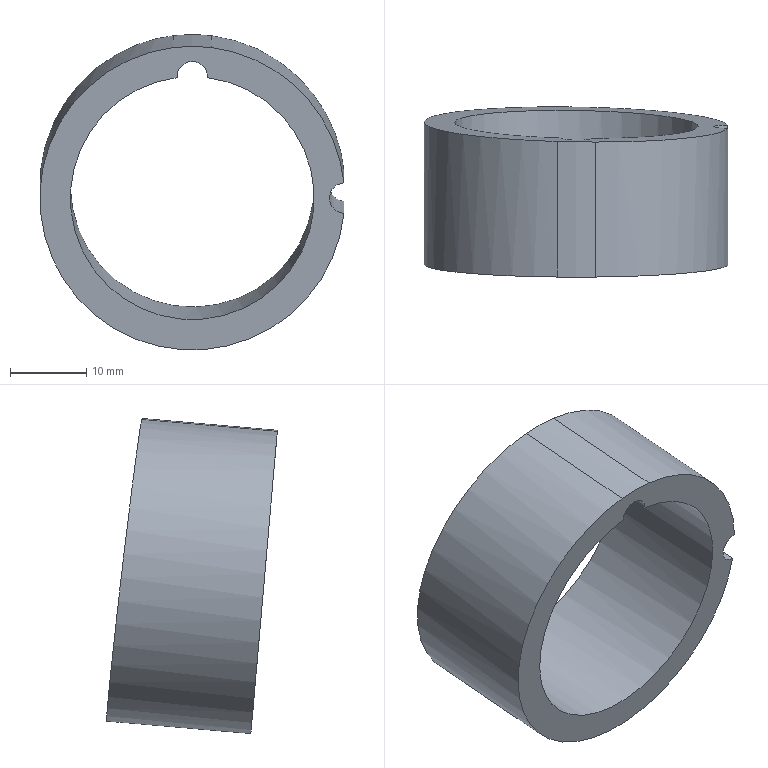Part | NX | features solid 2 | 1 solid | 8 faces | box 39.9 x 22.412 x 41.4 mm | volume 8096 mm3 | cylinder 5 | plane 2 | spline 1 | commonest cylinder face diameters 4 x2 40 x2 32 x1
STEP:
#1=CARTESIAN_POINT('',(191.232,38.007,-25.778));
#2=VERTEX_POINT('',#1);
#3=CARTESIAN_POINT('',(208.637,39.562,-43.556));
#4=VERTEX_POINT('',#3);
#5=CARTESIAN_POINT('',(188.737,39.736,-45.546));
#6=DIRECTION('',(0.,0.9962,0.08716));
#7=DIRECTION('',(0.,-0.08716,0.9962));
#8=AXIS2_PLACEMENT_3D('',#5,#6,#7);
#9=CIRCLE('',#8,20.);
#10=EDGE_CURVE('',#2,#4,#9,.T.);
#11=ORIENTED_EDGE('',*,*,#10,.T.);
#12=CARTESIAN_POINT('',(208.637,57.524,-41.984));
#13=VERTEX_POINT('',#12);
#14=CARTESIAN_POINT('',(208.637,48.658,-42.76));
#15=DIRECTION('',(0.,-0.9962,-0.08716));
#16=VECTOR('',#15,1000.);
#17=LINE('',#14,#16);
#18=EDGE_CURVE('',#4,#13,#17,.F.);
#19=ORIENTED_EDGE('',*,*,#18,.T.);
#20=CARTESIAN_POINT('',(191.232,55.721,-24.228));
#21=VERTEX_POINT('',#20);
#22=CARTESIAN_POINT('',(188.737,58.063,-43.942));
#23=DIRECTION('',(0.01549,0.9931,0.116));
#24=DIRECTION('',(0.4705,-0.1096,0.8755));
#25=AXIS2_PLACEMENT_3D('',#22,#23,#24);
#26=ELLIPSE('',#25,20.011,20.);
#27=EDGE_CURVE('',#21,#13,#26,.T.);
#28=ORIENTED_EDGE('',*,*,#27,.F.);
#29=CARTESIAN_POINT('',(191.232,57.931,-24.034));
#30=DIRECTION('',(0.,-0.9962,-0.08716));
#31=VECTOR('',#30,1000.);
#32=LINE('',#29,#31);
#33=EDGE_CURVE('',#21,#2,#32,.T.);
#34=ORIENTED_EDGE('',*,*,#33,.T.);
#35=EDGE_LOOP('',(#11,#19,#28,#34));
#36=FACE_BOUND('',#35,.T.);
#37=CARTESIAN_POINT('',(188.737,59.66,-43.803));
#38=DIRECTION('',(0.,-0.9962,-0.08716));
#39=DIRECTION('',(0.,0.08716,-0.9962));
#40=AXIS2_PLACEMENT_3D('',#37,#38,#39);
#41=CYLINDRICAL_SURFACE('',#40,20.);
#42=ADVANCED_FACE('',(#36),#41,.T.);
#43=CARTESIAN_POINT('',(190.733,38.353,-29.731));
#44=VERTEX_POINT('',#43);
#45=CARTESIAN_POINT('',(186.741,38.353,-29.731));
#46=VERTEX_POINT('',#45);
#47=CARTESIAN_POINT('',(188.737,39.736,-45.546));
#48=DIRECTION('',(0.,-0.9962,-0.08716));
#49=DIRECTION('',(0.,0.08716,-0.9962));
#50=AXIS2_PLACEMENT_3D('',#47,#48,#49);
#51=CIRCLE('',#50,16.);
#52=EDGE_CURVE('',#44,#46,#51,.F.);
#53=ORIENTED_EDGE('',*,*,#52,.F.);
#54=CARTESIAN_POINT('',(190.733,56.189,-28.171));
#55=VERTEX_POINT('',#54);
#56=CARTESIAN_POINT('',(190.733,58.277,-27.988));
#57=DIRECTION('',(0.,-0.9962,-0.08716));
#58=VECTOR('',#57,1000.);
#59=LINE('',#56,#58);
#60=EDGE_CURVE('',#44,#55,#59,.F.);
#61=ORIENTED_EDGE('',*,*,#60,.T.);
#62=CARTESIAN_POINT('',(186.741,56.251,-28.165));
#63=VERTEX_POINT('',#62);
#64=CARTESIAN_POINT('',(188.737,58.063,-43.942));
#65=DIRECTION('',(0.01549,0.9931,0.116));
#66=DIRECTION('',(0.4705,-0.1096,0.8755));
#67=AXIS2_PLACEMENT_3D('',#64,#65,#66);
#68=ELLIPSE('',#67,16.009,16.);
#69=EDGE_CURVE('',#55,#63,#68,.T.);
#70=ORIENTED_EDGE('',*,*,#69,.T.);
#71=CARTESIAN_POINT('',(186.741,58.277,-27.988));
#72=DIRECTION('',(0.,-0.9962,-0.08716));
#73=VECTOR('',#72,1000.);
#74=LINE('',#71,#73);
#75=EDGE_CURVE('',#63,#46,#74,.T.);
#76=ORIENTED_EDGE('',*,*,#75,.T.);
#77=EDGE_LOOP('',(#53,#61,#70,#76));
#78=FACE_BOUND('',#77,.T.);
#79=CARTESIAN_POINT('',(188.737,59.66,-43.803));
#80=DIRECTION('',(0.,-0.9962,-0.08716));
#81=DIRECTION('',(0.,0.08716,-0.9962));
#82=AXIS2_PLACEMENT_3D('',#79,#80,#81);
#83=CYLINDRICAL_SURFACE('',#82,16.);
#84=ADVANCED_FACE('',(#78),#83,.F.);
#85=CARTESIAN_POINT('',(208.637,57.988,-45.954));
#86=VERTEX_POINT('',#85);
#87=CARTESIAN_POINT('',(208.737,57.754,-43.969));
#88=DIRECTION('',(0.01549,0.9931,0.116));
#89=DIRECTION('',(0.4705,-0.1096,0.8755));
#90=AXIS2_PLACEMENT_3D('',#87,#88,#89);
#91=ELLIPSE('',#90,2.001,2.);
#92=EDGE_CURVE('',#86,#13,#91,.T.);
#93=ORIENTED_EDGE('',*,*,#92,.F.);
#94=CARTESIAN_POINT('',(186.242,55.798,-24.221));
#95=VERTEX_POINT('',#94);
#96=CARTESIAN_POINT('',(188.737,58.063,-43.942));
#97=DIRECTION('',(0.01549,0.9931,0.116));
#98=DIRECTION('',(0.4705,-0.1096,0.8755));
#99=AXIS2_PLACEMENT_3D('',#96,#97,#98);
#100=ELLIPSE('',#99,20.011,20.);
#101=EDGE_CURVE('',#86,#95,#100,.T.);
#102=ORIENTED_EDGE('',*,*,#101,.T.);
#103=CARTESIAN_POINT('',(186.242,55.798,-24.221));
#104=CARTESIAN_POINT('',(187.898,55.748,-24.016));
#105=CARTESIAN_POINT('',(189.576,55.722,-24.019));
#106=CARTESIAN_POINT('',(191.232,55.721,-24.228));
#107=B_SPLINE_CURVE_WITH_KNOTS('',3,(#103,#104,#105,#106),.UNSPECIFIED.,.F.,.F.,(4,4),(0.,0.005005),.UNSPECIFIED.);
#108=EDGE_CURVE('',#95,#21,#107,.T.);
#109=ORIENTED_EDGE('',*,*,#108,.T.);
#110=ORIENTED_EDGE('',*,*,#27,.T.);
#111=EDGE_LOOP('',(#93,#102,#109,#110));
#112=FACE_BOUND('',#111,.T.);
#113=CARTESIAN_POINT('',(188.737,56.206,-28.044));
#114=DIRECTION('',(0.01549,0.9931,0.116));
#115=DIRECTION('',(0.4705,-0.1096,0.8755));
#116=AXIS2_PLACEMENT_3D('',#113,#114,#115);
#117=ELLIPSE('',#116,2.001,2.);
#118=EDGE_CURVE('',#63,#55,#117,.T.);
#119=ORIENTED_EDGE('',*,*,#118,.F.);
#120=ORIENTED_EDGE('',*,*,#69,.F.);
#121=EDGE_LOOP('',(#119,#120));
#122=FACE_BOUND('',#121,.T.);
#123=CARTESIAN_POINT('',(159.246,62.921,-81.584));
#124=DIRECTION('',(0.01549,0.9931,0.116));
#125=DIRECTION('',(0.06594,-0.1168,0.991));
#126=AXIS2_PLACEMENT_3D('',#123,#124,#125);
#127=PLANE('',#126);
#128=ADVANCED_FACE('',(#112,#122),#127,.T.);
#129=CARTESIAN_POINT('',(208.637,39.91,-47.536));
#130=VERTEX_POINT('',#129);
#131=CARTESIAN_POINT('',(208.737,39.736,-45.546));
#132=DIRECTION('',(0.,-0.9962,-0.08716));
#133=DIRECTION('',(0.,0.08716,-0.9962));
#134=AXIS2_PLACEMENT_3D('',#131,#132,#133);
#135=CIRCLE('',#134,2.);
#136=EDGE_CURVE('',#4,#130,#135,.T.);
#137=ORIENTED_EDGE('',*,*,#136,.F.);
#138=ORIENTED_EDGE('',*,*,#10,.F.);
#139=CARTESIAN_POINT('',(186.242,38.007,-25.778));
#140=VERTEX_POINT('',#139);
#141=CARTESIAN_POINT('',(186.242,38.007,-25.778));
#142=CARTESIAN_POINT('',(187.899,37.989,-25.57));
#143=CARTESIAN_POINT('',(189.575,37.989,-25.57));
#144=CARTESIAN_POINT('',(191.232,38.007,-25.778));
#145=B_SPLINE_CURVE_WITH_KNOTS('',3,(#141,#142,#143,#144),.UNSPECIFIED.,.F.,.F.,(4,4),(0.,1.),.PIECEWISE_BEZIER_KNOTS.);
#146=EDGE_CURVE('',#140,#2,#145,.T.);
#147=ORIENTED_EDGE('',*,*,#146,.F.);
#148=CARTESIAN_POINT('',(188.737,39.736,-45.546));
#149=DIRECTION('',(0.,0.9962,0.08716));
#150=DIRECTION('',(0.,-0.08716,0.9962));
#151=AXIS2_PLACEMENT_3D('',#148,#149,#150);
#152=CIRCLE('',#151,20.);
#153=EDGE_CURVE('',#130,#140,#152,.T.);
#154=ORIENTED_EDGE('',*,*,#153,.F.);
#155=EDGE_LOOP('',(#137,#138,#147,#154));
#156=FACE_BOUND('',#155,.T.);
#157=CARTESIAN_POINT('',(188.737,38.342,-29.607));
#158=DIRECTION('',(0.,-0.9962,-0.08716));
#159=DIRECTION('',(0.,0.08716,-0.9962));
#160=AXIS2_PLACEMENT_3D('',#157,#158,#159);
#161=CIRCLE('',#160,2.);
#162=EDGE_CURVE('',#44,#46,#161,.T.);
#163=ORIENTED_EDGE('',*,*,#162,.F.);
#164=ORIENTED_EDGE('',*,*,#52,.T.);
#165=EDGE_LOOP('',(#163,#164));
#166=FACE_BOUND('',#165,.T.);
#167=CARTESIAN_POINT('',(186.242,38.007,-25.778));
#168=DIRECTION('',(0.,0.9962,0.08716));
#169=DIRECTION('',(0.,-0.08716,0.9962));
#170=AXIS2_PLACEMENT_3D('',#167,#168,#169);
#171=PLANE('',#170);
#172=ADVANCED_FACE('',(#156,#166),#171,.F.);
#173=ORIENTED_EDGE('',*,*,#101,.F.);
#174=CARTESIAN_POINT('',(208.637,49.007,-46.74));
#175=DIRECTION('',(0.,-0.9962,-0.08716));
#176=VECTOR('',#175,1000.);
#177=LINE('',#174,#176);
#178=EDGE_CURVE('',#86,#130,#177,.T.);
#179=ORIENTED_EDGE('',*,*,#178,.T.);
#180=ORIENTED_EDGE('',*,*,#153,.T.);
#181=CARTESIAN_POINT('',(186.242,57.931,-24.034));
#182=DIRECTION('',(0.,-0.9962,-0.08716));
#183=VECTOR('',#182,1000.);
#184=LINE('',#181,#183);
#185=EDGE_CURVE('',#95,#140,#184,.T.);
#186=ORIENTED_EDGE('',*,*,#185,.F.);
#187=EDGE_LOOP('',(#173,#179,#180,#186));
#188=FACE_BOUND('',#187,.T.);
#189=CARTESIAN_POINT('',(188.737,59.66,-43.803));
#190=DIRECTION('',(0.,-0.9962,-0.08716));
#191=DIRECTION('',(0.,0.08716,-0.9962));
#192=AXIS2_PLACEMENT_3D('',#189,#190,#191);
#193=CYLINDRICAL_SURFACE('',#192,20.);
#194=ADVANCED_FACE('',(#188),#193,.T.);
#195=ORIENTED_EDGE('',*,*,#146,.T.);
#196=ORIENTED_EDGE('',*,*,#33,.F.);
#197=ORIENTED_EDGE('',*,*,#108,.F.);
#198=ORIENTED_EDGE('',*,*,#185,.T.);
#199=EDGE_LOOP('',(#195,#196,#197,#198));
#200=FACE_BOUND('',#199,.T.);
#201=CARTESIAN_POINT('',(186.242,55.905,-24.212));
#202=CARTESIAN_POINT('',(186.242,38.007,-25.778));
#203=CARTESIAN_POINT('',(187.899,55.887,-24.004));
#204=CARTESIAN_POINT('',(187.899,37.989,-25.57));
#205=CARTESIAN_POINT('',(189.575,55.887,-24.004));
#206=CARTESIAN_POINT('',(189.575,37.989,-25.57));
#207=CARTESIAN_POINT('',(191.232,55.905,-24.212));
#208=CARTESIAN_POINT('',(191.232,38.007,-25.778));
#209=B_SPLINE_SURFACE_WITH_KNOTS('',3,1,((#201,#202),(#203,#204),(#205,#206),(#207,#208)),.SURF_OF_LINEAR_EXTRUSION.,.F.,.F.,.F.,(4,4),(2,2),(0.,1.),(0.,1.),.PIECEWISE_BEZIER_KNOTS.);
#210=ADVANCED_FACE('',(#200),#209,.F.);
#211=ORIENTED_EDGE('',*,*,#75,.F.);
#212=ORIENTED_EDGE('',*,*,#118,.T.);
#213=ORIENTED_EDGE('',*,*,#60,.F.);
#214=ORIENTED_EDGE('',*,*,#162,.T.);
#215=EDGE_LOOP('',(#211,#212,#213,#214));
#216=FACE_BOUND('',#215,.T.);
#217=CARTESIAN_POINT('',(188.737,58.266,-27.864));
#218=DIRECTION('',(0.,-0.9962,-0.08716));
#219=DIRECTION('',(0.,-0.08716,0.9962));
#220=AXIS2_PLACEMENT_3D('',#217,#218,#219);
#221=CYLINDRICAL_SURFACE('',#220,2.);
#222=ADVANCED_FACE('',(#216),#221,.F.);
#223=ORIENTED_EDGE('',*,*,#136,.T.);
#224=ORIENTED_EDGE('',*,*,#178,.F.);
#225=ORIENTED_EDGE('',*,*,#92,.T.);
#226=ORIENTED_EDGE('',*,*,#18,.F.);
#227=EDGE_LOOP('',(#223,#224,#225,#226));
#228=FACE_BOUND('',#227,.T.);
#229=CARTESIAN_POINT('',(208.737,59.66,-43.803));
#230=DIRECTION('',(0.,-0.9962,-0.08716));
#231=DIRECTION('',(0.,-0.08716,0.9962));
#232=AXIS2_PLACEMENT_3D('',#229,#230,#231);
#233=CYLINDRICAL_SURFACE('',#232,2.);
#234=ADVANCED_FACE('',(#228),#233,.F.);
#235=CLOSED_SHELL('',(#42,#84,#128,#172,#194,#210,#222,#234));
#236=MANIFOLD_SOLID_BREP('',#235);
#237=(LENGTH_UNIT()NAMED_UNIT(*)SI_UNIT(.MILLI.,.METRE.));
#238=UNCERTAINTY_MEASURE_WITH_UNIT(LENGTH_MEASURE(0.0508),#237,'','');
#239=(NAMED_UNIT(*)PLANE_ANGLE_UNIT()SI_UNIT($,.RADIAN.));
#240=(NAMED_UNIT(*)SI_UNIT($,.STERADIAN.)SOLID_ANGLE_UNIT());
#241=(GEOMETRIC_REPRESENTATION_CONTEXT(3)GLOBAL_UNCERTAINTY_ASSIGNED_CONTEXT((#238))GLOBAL_UNIT_ASSIGNED_CONTEXT((#237,#239,#240))REPRESENTATION_CONTEXT('',''));
#242=ADVANCED_BREP_SHAPE_REPRESENTATION('',(#236),#241);